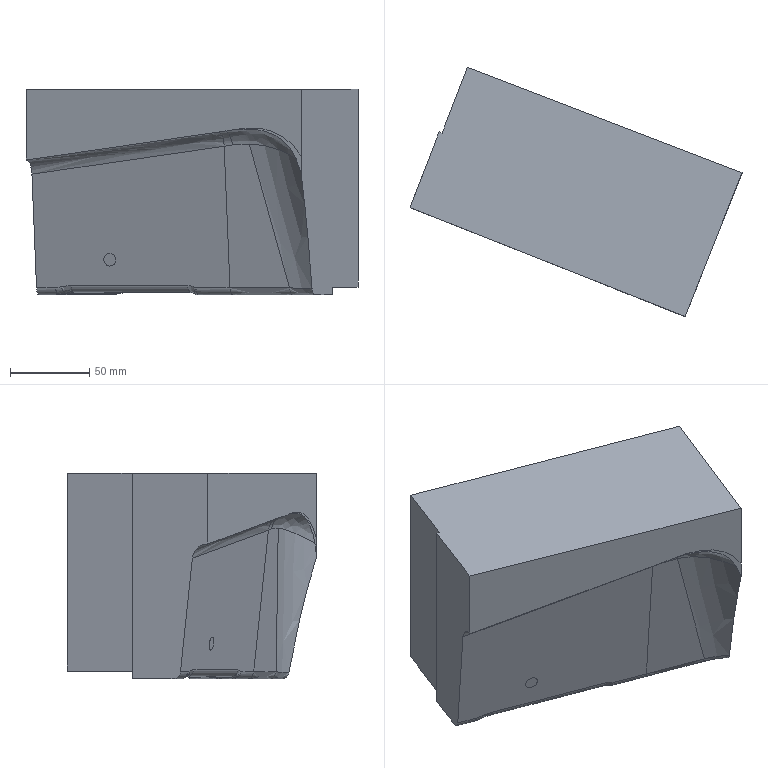Part | NX | features solid 2 | 1 solid | 52 faces | box 209.361 x 157.25 x 129.85 mm | volume 2031445 mm3 | spline 45 | plane 7